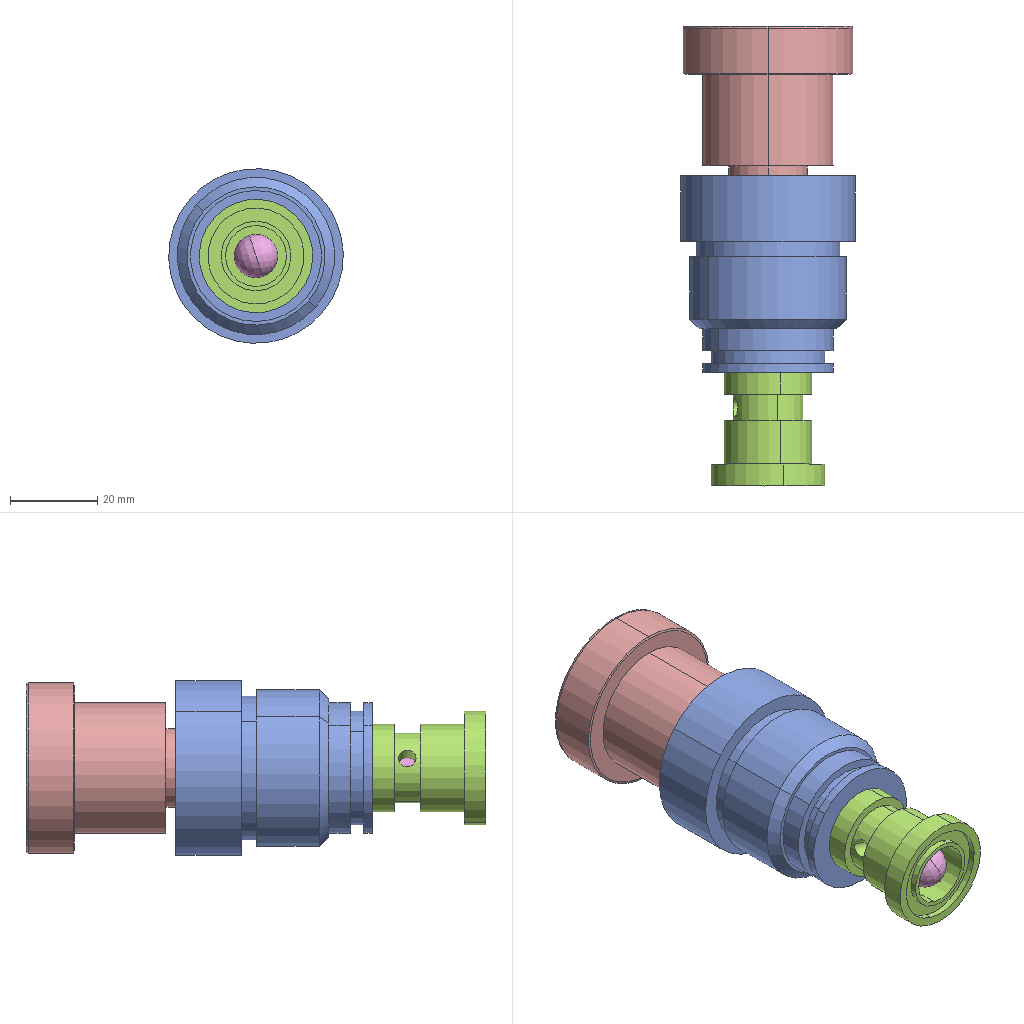Assembly | SolidWorks | 5 different items | 5 placed | box 40 x 105 x 40 mm
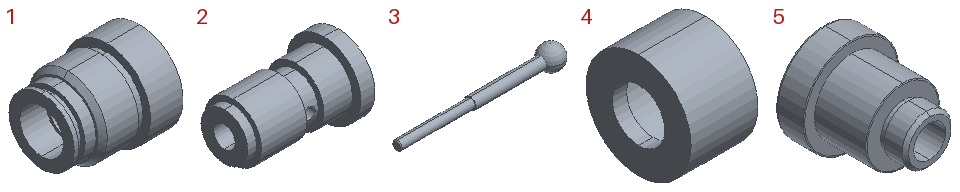Parts list (item | quantity | size | volume | features):
1 | x1 | 45 x 40 x 40 mm | 33217 mm3 | features ICE 8, Extrusion 1, HoleWzd 1, StudWizard 1
2 | x1 | 40 x 26 x 26 mm | 9972 mm3 | features ICE 5, Cut 1, Extrusion 1, RevCut 1, SweepCut 1
3 | x1 | 72 x 10 x 10 mm | 1520 mm3 | features Extrusion 1, Revolution 1, StudWizard 1
4 | x1 | 7 x 11 x 11 mm | 317.497 mm3 | features Extrusion 1, ICE 1
5 | x1 | 39 x 43 x 39 mm | 27675 mm3 | features ICE 4, Chamfer 2, Extrusion 1, StudWizard 1
Mates (type | each side: item.copy, entity, surface, feature):
Concentric | 5.1 face cylinder Cut-Extrude1 | 3.1 face cylinder Boss-Extrude1
Concentric | 5.1 face cylinder Boss-Extrude3 | 1.1 face cylinder Boss-Extrude6
Concentric | 1.1 face cylinder Cut-Extrude1 | 2.1 face cylinder Boss-Extrude2
Concentric | 1.1 face cylinder Cut-Extrude1 | 4.1 face cylinder Boss-Extrude1
Coincident | 5.1 face plane Boss-Extrude1 | 1.1 face plane Boss-Extrude6
Tangent | 2.1 face plane Cut-Extrude1 | 3.1 face sphere Revolve1
DistanceDim | 1.1 face plane Boss-Extrude1 | 2.1 face plane Cut-Revolve1